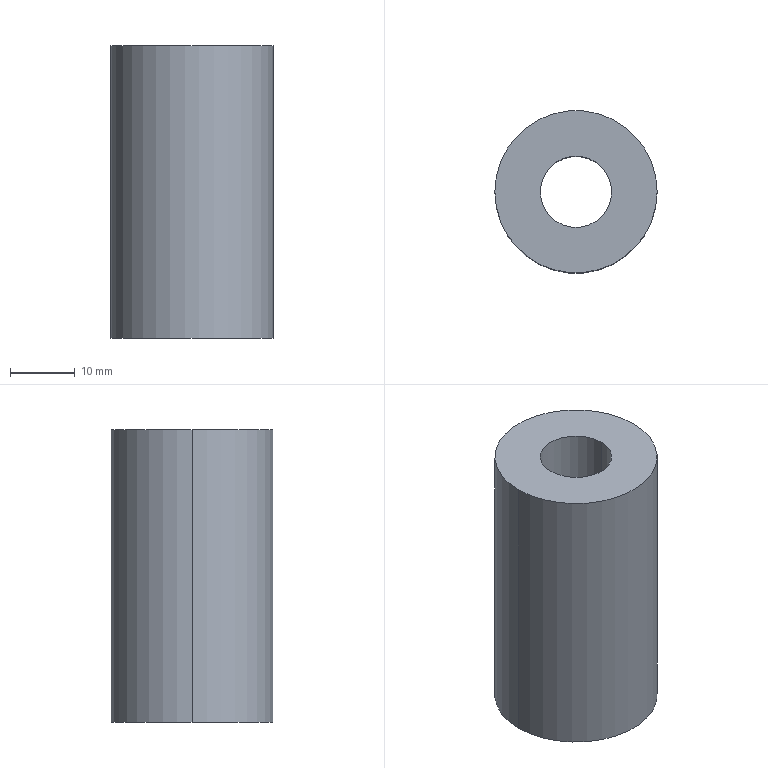Part | 1 solid | 6 faces | box 25 x 25 x 45 mm | volume 17813 mm3 | cylinder 4 | plane 2 | commonest cylinder face diameters 11 x2 25 x2
STEP:
#1=CARTESIAN_POINT('',(5.5,0.,45.));
#2=VERTEX_POINT('',#1);
#3=CARTESIAN_POINT('',(-5.5,0.,45.));
#4=VERTEX_POINT('',#3);
#5=CARTESIAN_POINT('',(0.,0.,45.));
#6=DIRECTION('',(0.,0.,-1.));
#7=DIRECTION('',(-1.,0.,0.));
#8=AXIS2_PLACEMENT_3D('',#5,#6,#7);
#9=CIRCLE('',#8,5.5);
#10=EDGE_CURVE('',#2,#4,#9,.T.);
#11=ORIENTED_EDGE('',*,*,#10,.F.);
#12=CARTESIAN_POINT('',(5.5,0.,0.));
#13=VERTEX_POINT('',#12);
#14=CARTESIAN_POINT('',(5.5,0.,0.));
#15=DIRECTION('',(0.,0.,-1.));
#16=VECTOR('',#15,1000.);
#17=LINE('',#14,#16);
#18=EDGE_CURVE('',#2,#13,#17,.T.);
#19=ORIENTED_EDGE('',*,*,#18,.T.);
#20=CARTESIAN_POINT('',(-5.5,0.,0.));
#21=VERTEX_POINT('',#20);
#22=CARTESIAN_POINT('',(0.,0.,0.));
#23=DIRECTION('',(0.,0.,-1.));
#24=DIRECTION('',(-1.,0.,0.));
#25=AXIS2_PLACEMENT_3D('',#22,#23,#24);
#26=CIRCLE('',#25,5.5);
#27=EDGE_CURVE('',#13,#21,#26,.T.);
#28=ORIENTED_EDGE('',*,*,#27,.T.);
#29=CARTESIAN_POINT('',(-5.5,0.,0.));
#30=DIRECTION('',(0.,0.,-1.));
#31=VECTOR('',#30,1000.);
#32=LINE('',#29,#31);
#33=EDGE_CURVE('',#4,#21,#32,.T.);
#34=ORIENTED_EDGE('',*,*,#33,.F.);
#35=EDGE_LOOP('',(#11,#19,#28,#34));
#36=FACE_OUTER_BOUND('',#35,.T.);
#37=CARTESIAN_POINT('',(0.,0.,0.));
#38=DIRECTION('',(0.,0.,-1.));
#39=DIRECTION('',(-1.,0.,0.));
#40=AXIS2_PLACEMENT_3D('',#37,#38,#39);
#41=CYLINDRICAL_SURFACE('',#40,5.5);
#42=ADVANCED_FACE('',(#36),#41,.F.);
#43=CARTESIAN_POINT('',(12.5,0.,45.));
#44=VERTEX_POINT('',#43);
#45=CARTESIAN_POINT('',(-12.5,0.,45.));
#46=VERTEX_POINT('',#45);
#47=CARTESIAN_POINT('',(0.,0.,45.));
#48=DIRECTION('',(0.,0.,1.));
#49=DIRECTION('',(1.,0.,0.));
#50=AXIS2_PLACEMENT_3D('',#47,#48,#49);
#51=CIRCLE('',#50,12.5);
#52=EDGE_CURVE('',#44,#46,#51,.T.);
#53=ORIENTED_EDGE('',*,*,#52,.F.);
#54=CARTESIAN_POINT('',(12.5,0.,0.));
#55=VERTEX_POINT('',#54);
#56=CARTESIAN_POINT('',(12.5,0.,25.));
#57=DIRECTION('',(0.,0.,-1.));
#58=VECTOR('',#57,1000.);
#59=LINE('',#56,#58);
#60=EDGE_CURVE('',#44,#55,#59,.T.);
#61=ORIENTED_EDGE('',*,*,#60,.T.);
#62=CARTESIAN_POINT('',(-12.5,0.,0.));
#63=VERTEX_POINT('',#62);
#64=CARTESIAN_POINT('',(0.,0.,0.));
#65=DIRECTION('',(0.,0.,1.));
#66=DIRECTION('',(1.,0.,0.));
#67=AXIS2_PLACEMENT_3D('',#64,#65,#66);
#68=CIRCLE('',#67,12.5);
#69=EDGE_CURVE('',#55,#63,#68,.T.);
#70=ORIENTED_EDGE('',*,*,#69,.T.);
#71=CARTESIAN_POINT('',(-12.5,0.,25.));
#72=DIRECTION('',(0.,0.,-1.));
#73=VECTOR('',#72,1000.);
#74=LINE('',#71,#73);
#75=EDGE_CURVE('',#46,#63,#74,.T.);
#76=ORIENTED_EDGE('',*,*,#75,.F.);
#77=EDGE_LOOP('',(#53,#61,#70,#76));
#78=FACE_OUTER_BOUND('',#77,.T.);
#79=CARTESIAN_POINT('',(0.,0.,25.));
#80=DIRECTION('',(0.,0.,-1.));
#81=DIRECTION('',(-1.,0.,0.));
#82=AXIS2_PLACEMENT_3D('',#79,#80,#81);
#83=CYLINDRICAL_SURFACE('',#82,12.5);
#84=ADVANCED_FACE('',(#78),#83,.T.);
#85=ORIENTED_EDGE('',*,*,#60,.F.);
#86=CARTESIAN_POINT('',(0.,0.,45.));
#87=DIRECTION('',(0.,0.,1.));
#88=DIRECTION('',(1.,0.,0.));
#89=AXIS2_PLACEMENT_3D('',#86,#87,#88);
#90=CIRCLE('',#89,12.5);
#91=EDGE_CURVE('',#46,#44,#90,.T.);
#92=ORIENTED_EDGE('',*,*,#91,.F.);
#93=ORIENTED_EDGE('',*,*,#75,.T.);
#94=CARTESIAN_POINT('',(0.,0.,0.));
#95=DIRECTION('',(0.,0.,1.));
#96=DIRECTION('',(1.,0.,0.));
#97=AXIS2_PLACEMENT_3D('',#94,#95,#96);
#98=CIRCLE('',#97,12.5);
#99=EDGE_CURVE('',#63,#55,#98,.T.);
#100=ORIENTED_EDGE('',*,*,#99,.T.);
#101=EDGE_LOOP('',(#85,#92,#93,#100));
#102=FACE_OUTER_BOUND('',#101,.T.);
#103=CARTESIAN_POINT('',(0.,0.,25.));
#104=DIRECTION('',(0.,0.,-1.));
#105=DIRECTION('',(-1.,0.,0.));
#106=AXIS2_PLACEMENT_3D('',#103,#104,#105);
#107=CYLINDRICAL_SURFACE('',#106,12.5);
#108=ADVANCED_FACE('',(#102),#107,.T.);
#109=CARTESIAN_POINT('',(0.,0.,0.));
#110=DIRECTION('',(0.,0.,-1.));
#111=DIRECTION('',(-1.,0.,0.));
#112=AXIS2_PLACEMENT_3D('',#109,#110,#111);
#113=CIRCLE('',#112,5.5);
#114=EDGE_CURVE('',#21,#13,#113,.T.);
#115=ORIENTED_EDGE('',*,*,#114,.F.);
#116=ORIENTED_EDGE('',*,*,#27,.F.);
#117=EDGE_LOOP('',(#115,#116));
#118=FACE_BOUND('',#117,.T.);
#119=ORIENTED_EDGE('',*,*,#99,.F.);
#120=ORIENTED_EDGE('',*,*,#69,.F.);
#121=EDGE_LOOP('',(#119,#120));
#122=FACE_OUTER_BOUND('',#121,.T.);
#123=CARTESIAN_POINT('',(0.,0.,0.));
#124=DIRECTION('',(0.,0.,1.));
#125=DIRECTION('',(1.,0.,0.));
#126=AXIS2_PLACEMENT_3D('',#123,#124,#125);
#127=PLANE('',#126);
#128=ADVANCED_FACE('',(#118,#122),#127,.F.);
#129=CARTESIAN_POINT('',(0.,0.,45.));
#130=DIRECTION('',(0.,0.,-1.));
#131=DIRECTION('',(-1.,0.,0.));
#132=AXIS2_PLACEMENT_3D('',#129,#130,#131);
#133=CIRCLE('',#132,5.5);
#134=EDGE_CURVE('',#4,#2,#133,.T.);
#135=ORIENTED_EDGE('',*,*,#134,.T.);
#136=ORIENTED_EDGE('',*,*,#10,.T.);
#137=EDGE_LOOP('',(#135,#136));
#138=FACE_BOUND('',#137,.T.);
#139=ORIENTED_EDGE('',*,*,#91,.T.);
#140=ORIENTED_EDGE('',*,*,#52,.T.);
#141=EDGE_LOOP('',(#139,#140));
#142=FACE_OUTER_BOUND('',#141,.T.);
#143=CARTESIAN_POINT('',(0.,0.,45.));
#144=DIRECTION('',(0.,0.,1.));
#145=DIRECTION('',(1.,0.,0.));
#146=AXIS2_PLACEMENT_3D('',#143,#144,#145);
#147=PLANE('',#146);
#148=ADVANCED_FACE('',(#138,#142),#147,.T.);
#149=ORIENTED_EDGE('',*,*,#18,.F.);
#150=ORIENTED_EDGE('',*,*,#134,.F.);
#151=ORIENTED_EDGE('',*,*,#33,.T.);
#152=ORIENTED_EDGE('',*,*,#114,.T.);
#153=EDGE_LOOP('',(#149,#150,#151,#152));
#154=FACE_OUTER_BOUND('',#153,.T.);
#155=CARTESIAN_POINT('',(0.,0.,0.));
#156=DIRECTION('',(0.,0.,-1.));
#157=DIRECTION('',(-1.,0.,0.));
#158=AXIS2_PLACEMENT_3D('',#155,#156,#157);
#159=CYLINDRICAL_SURFACE('',#158,5.5);
#160=ADVANCED_FACE('',(#154),#159,.F.);
#161=CLOSED_SHELL('',(#42,#84,#108,#128,#148,#160));
#162=MANIFOLD_SOLID_BREP('',#161);
#163=CARTESIAN_POINT('',(0.,0.,0.));
#164=DIRECTION('',(0.,0.,1.));
#165=DIRECTION('',(1.,0.,0.));
#166=AXIS2_PLACEMENT_3D('',#163,#164,#165);
#167=(LENGTH_UNIT()NAMED_UNIT(*)SI_UNIT(.MILLI.,.METRE.));
#168=UNCERTAINTY_MEASURE_WITH_UNIT(LENGTH_MEASURE(0.00001),#167,'','');
#169=(NAMED_UNIT(*)PLANE_ANGLE_UNIT()SI_UNIT($,.RADIAN.));
#170=(NAMED_UNIT(*)SI_UNIT($,.STERADIAN.)SOLID_ANGLE_UNIT());
#171=(GEOMETRIC_REPRESENTATION_CONTEXT(3)GLOBAL_UNCERTAINTY_ASSIGNED_CONTEXT((#168))GLOBAL_UNIT_ASSIGNED_CONTEXT((#167,#169,#170))REPRESENTATION_CONTEXT('',''));
#172=ADVANCED_BREP_SHAPE_REPRESENTATION('',(#162,#166),#171);